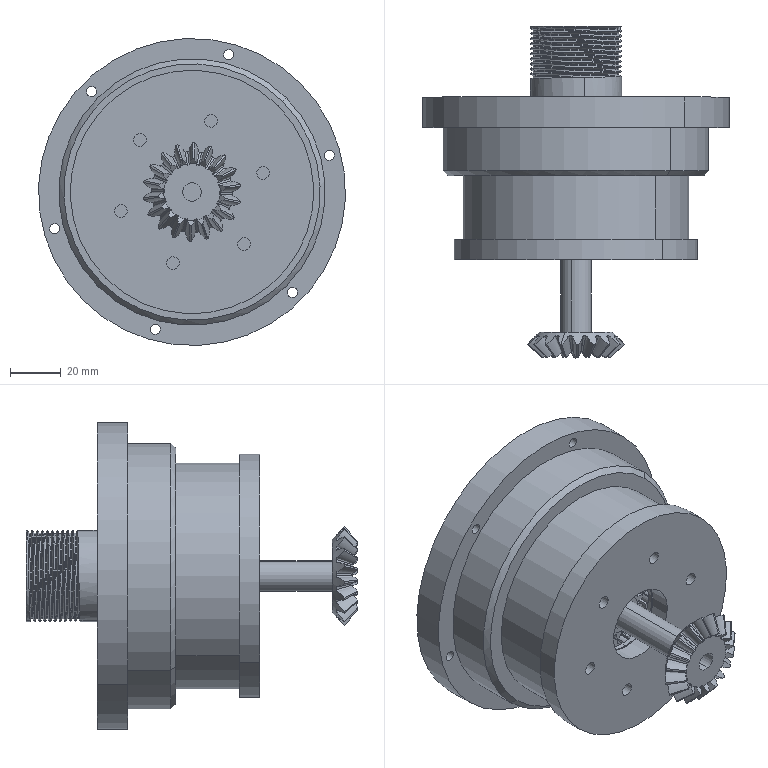Part | SolidWorks | features CompositeCurve 2 | 26 solids | 1796 faces | box 121 x 130.788 x 121 mm | volume 395483 mm3 | cylinder 757 | spline 651 | plane 346 | cone 42 | commonest cylinder face diameters 24.125 x57 29.25 x57 83.25 x57 69.75 x55 18.5 x54 22.5 x54